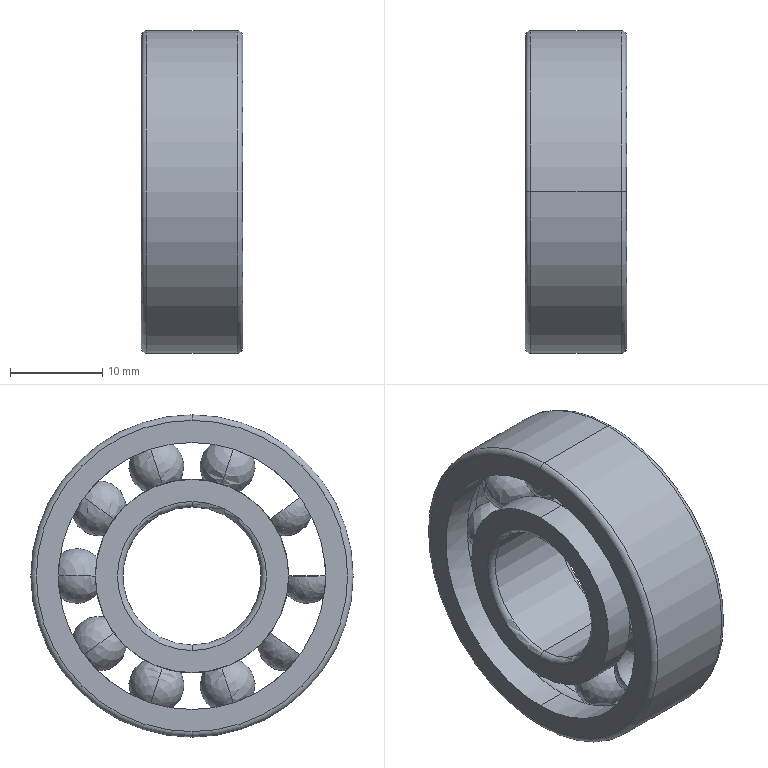Part | NX | features solid 2 | 1 solid | 77 faces | box 11 x 35 x 35 mm | volume 5484 mm3 | torus 41 | sphere 20 | cylinder 12 | plane 4 | commonest cylinder face diameters 21 x4 29 x4 15 x2 35 x2